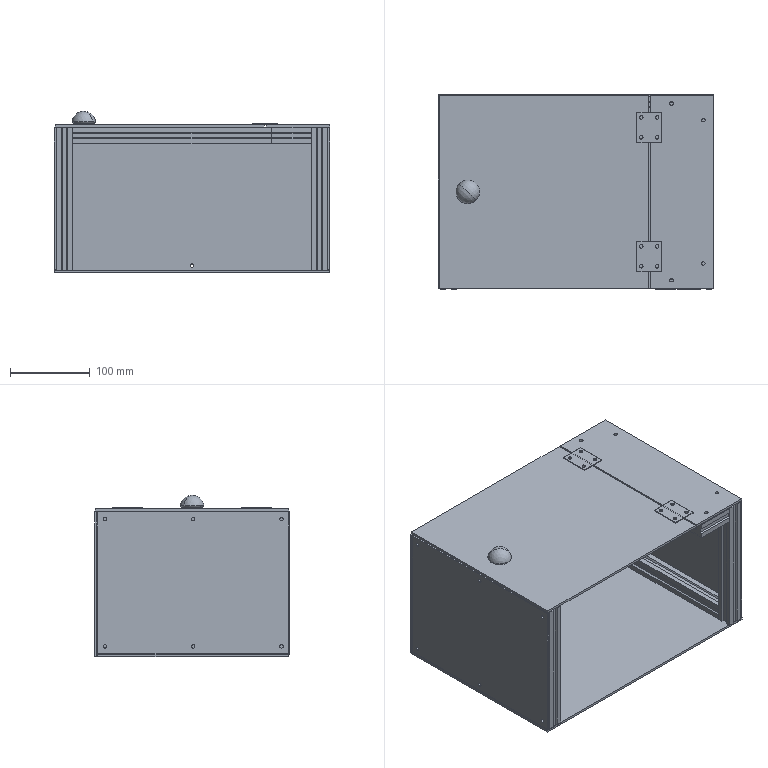Part | SolidWorks | features CompositeCurve 1 | 19 solids | 382 faces | box 346 x 245 x 203 mm | volume 1584731 mm3 | plane 270 | cylinder 108 | torus 2 | sphere 2 | commonest cylinder face diameters 4.4 x68 3.889 x20 4.5 x16 6.6 x2 10 x2